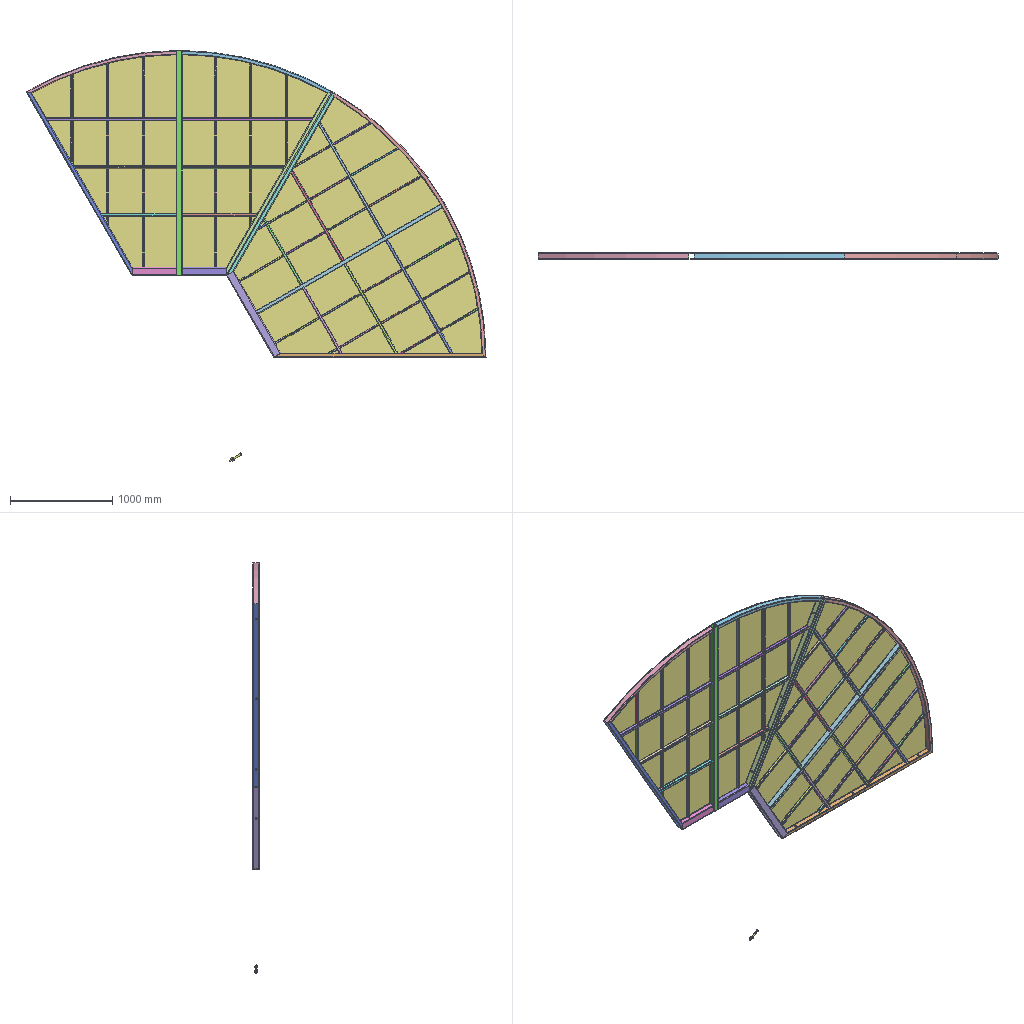Assembly | SolidWorks | 9 different items | 26 placed | box 4500 x 63 x 4020 mm
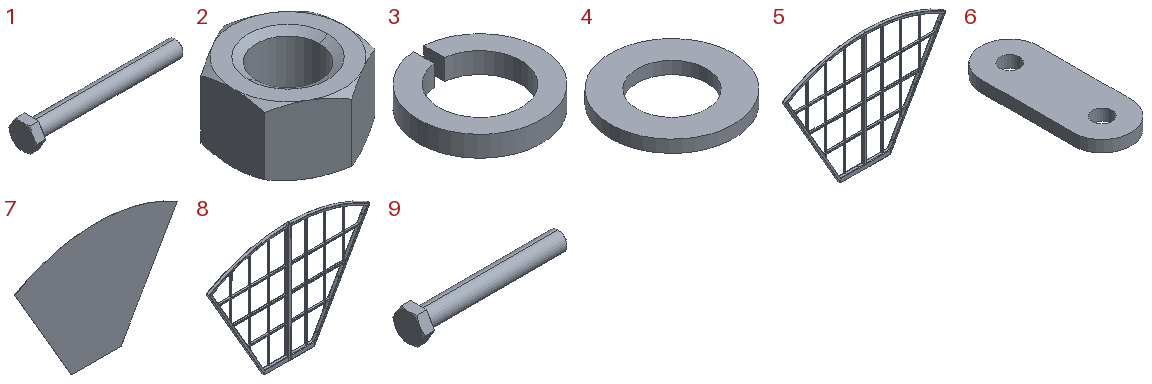Parts list (item | quantity | size | volume | features):
1 | x2 | 150 x 27.713 x 24 mm | 33047 mm3 | features Chamfer 2, RevCut 2, Revolution 2, Extrusion 1, ICE 1
2 | x5 | 24 x 27.713 x 14.8 mm | 5046 mm3 | features ICE 2, RevCut 2, Extrusion 1
3 | x5 | 24.356 x 24.313 x 4.1 mm | 1031 mm3 | features Extrusion 1
4 | x5 | 30 x 30 x 3 mm | 1440 mm3 | features Extrusion 1
5 | x1 | 3000 x 60 x 2200 mm | 9883837 mm3 | features WeldCornerFeat 7, WeldMemberFeat 4, HoleWzd 2, MirrorPattern 1, MirrorSolid 1, WeldmentFeature 1
6 | x2 | 50 x 130 x 10 mm | 55095 mm3 | features Extrusion 1
7 | x2 | 3000 x 3 x 2200 mm | 13028079 mm3 | features Extrusion 1
8 | x1 | 3000 x 60 x 2200 mm | 10098660 mm3 | features WeldCornerFeat 7, WeldMemberFeat 5, HoleWzd 2, MirrorPattern 1, MirrorSolid 1, WeldmentFeature 1
9 | x3 | 130 x 27.713 x 24 mm | 29026 mm3 | features Chamfer 2, RevCut 2, Revolution 2, Extrusion 1, ICE 1
Mates (type | each side: item.copy, entity, surface, feature):
Concentric | 2.1 face cylinder Boss-Extrude1 | 4.1 face cylinder Extrude1
Concentric | 4.1 face cylinder Extrude1 | 3.1 face cylinder Extrude1
Coincident | 4.1 face plane Extrude1 | 3.1 face plane Extrude1
Coincident | 2.1 face plane Boss-Extrude1 | 3.1 face plane Extrude1
Concentric | 9.1 face cylinder Revolve1 | 4.1 face cylinder Extrude1
Coincident | 5.1 face plane Gb/t 6728—2002 Rectangular hollow section 80X60X4(1) | 7.1 face plane Boss-Extrude1 | 2 times
Coincident | 5.1 face plane Gb/t 6728—2002 Rectangular hollow section 60X40X3(1) | 7.1 face plane Boss-Extrude1
Concentric | 5.1 face cylinder Ø17.0 (17) Diameter Hole2 | 9.2 face cylinder Revolve1
Coincident | 5.1 face plane Gb/t 6728—2002 Rectangular hollow section 80X60X4(1) | 9.2 face plane Boss-Extrude1
Coincident | 5.1 face plane Gb/t 6728—2002 Rectangular hollow section 80X60X4(1) | 6.1 face plane Boss-Extrude1
Parallel | 5.1 face plane Gb/t 6728—2002 Rectangular hollow section 60X40X3(1) | 6.1 face plane Boss-Extrude1
Concentric | 6.1 face cylinder Boss-Extrude1 | 9.2 face cylinder Revolve1
Concentric | 6.1 face cylinder Boss-Extrude1 | 1.1 face cylinder Revolve1
Coincident | 6.1 face plane Boss-Extrude1 | 4.2 face plane Extrude1
Coincident | 6.1 face plane Boss-Extrude1 | 4.3 face plane Extrude1
Concentric | 3.2 face cylinder Extrude1 | 9.2 face cylinder Revolve1
Coincident | 3.2 edge | 4.3 face plane Extrude1
Coincident | 3.2 face plane Extrude1 | 2.2 face plane Boss-Extrude1
Concentric | 4.3 face cylinder Extrude1 | 9.2 face cylinder Revolve1 | 2 times
Concentric | 2.2 face cylinder Boss-Extrude1 | 9.2 face cylinder Revolve1
Coincident | 9.2 face plane Revolve1 | 1.1 face plane Revolve1
Concentric | 3.3 face cylinder Extrude1 | 1.1 face cylinder Revolve1
Coincident | 3.3 face plane Extrude1 | 4.2 face plane Extrude1
Coincident | 3.3 face plane Extrude1 | 2.3 face plane Boss-Extrude1
Concentric | 1.1 face cylinder Revolve1 | 2.3 face cylinder Boss-Extrude1
Concentric | 1.1 face cylinder Revolve1 | 4.2 face cylinder Extrude1
Concentric | 8.1 face cylinder Ø17.0 (17) Diameter Hole2 | 6.2 face cylinder Boss-Extrude1
Coincident | 8.1 face plane Gb/t 6728—2002 Rectangular hollow section 80X60X4(1) | 6.2 face plane Boss-Extrude1
Parallel | 8.1 face plane Gb/t 6728—2002 Square hollow section 60×3-example.com(1) | 6.2 face plane Boss-Extrude1
Concentric | 8.1 face cylinder Ø17.0 (17) Diameter Hole2 | 9.3 face cylinder Revolve1
Coincident | 8.1 face plane Gb/t 6728—2002 Rectangular hollow section 80X60X4(1) | 9.3 face plane Boss-Extrude1
Coincident | 8.1 face plane Gb/t 6728—2002 Rectangular hollow section 60X40X3(1) | 7.2 face plane Boss-Extrude1
Coincident | 8.1 face plane Gb/t 6728—2002 Rectangular hollow section 80X60X4(1) | 7.2 face plane Boss-Extrude1
Coincident | 6.2 face plane Boss-Extrude1 | 4.4 face plane Extrude1
Concentric | 6.2 face cylinder Boss-Extrude1 | 1.2 face cylinder Revolve1
Concentric | 3.4 face cylinder Extrude1 | 9.3 face cylinder Revolve1
Coincident | 3.4 face plane Extrude1 | 4.4 face plane Extrude1
Coincident | 3.4 face plane Extrude1 | 2.4 face plane Boss-Extrude1
Concentric | 4.4 face cylinder Extrude1 | 9.3 face cylinder Revolve1
Concentric | 2.4 face cylinder Boss-Extrude1 | 9.3 face cylinder Revolve1
Coincident | 2.4 face plane Boss-Extrude1 | 2.5 face plane Boss-Extrude1
Coincident | 9.3 face plane Revolve1 | 1.2 face plane Revolve1
Concentric | 3.5 face cylinder Extrude1 | 1.2 face cylinder Revolve1
Coincident | 3.5 face plane Extrude1 | 2.5 face plane Boss-Extrude1
Coincident | 3.5 face plane Extrude1 | 4.5 face plane Extrude1
Concentric | 1.2 face cylinder Revolve1 | 4.5 face cylinder Extrude1
Concentric | 1.2 face cylinder Revolve1 | 2.5 face cylinder Boss-Extrude1
Concentric | 8.1 face cylinder Gb/t 6728—2002 Rectangular hollow section 60X40X3(1) | assembly axis
Concentric | 8.1 face cylinder Gb/t 6728—2002 Rectangular hollow section 60X40X3(1) | 5.1 face cylinder Gb/t 6728—2002 Rectangular hollow section 60X40X3(1)
Coincident | 5.1 face plane Gb/t 6728—2002 Rectangular hollow section 60X40X3(1) | 8.1 face plane Gb/t 6728—2002 Rectangular hollow section 60X40X3(1)
Coincident | 7.2 face plane Boss-Extrude1 | assembly plane
Coincident | 7.2 face plane Boss-Extrude1 | 7.1 face plane Boss-Extrude1